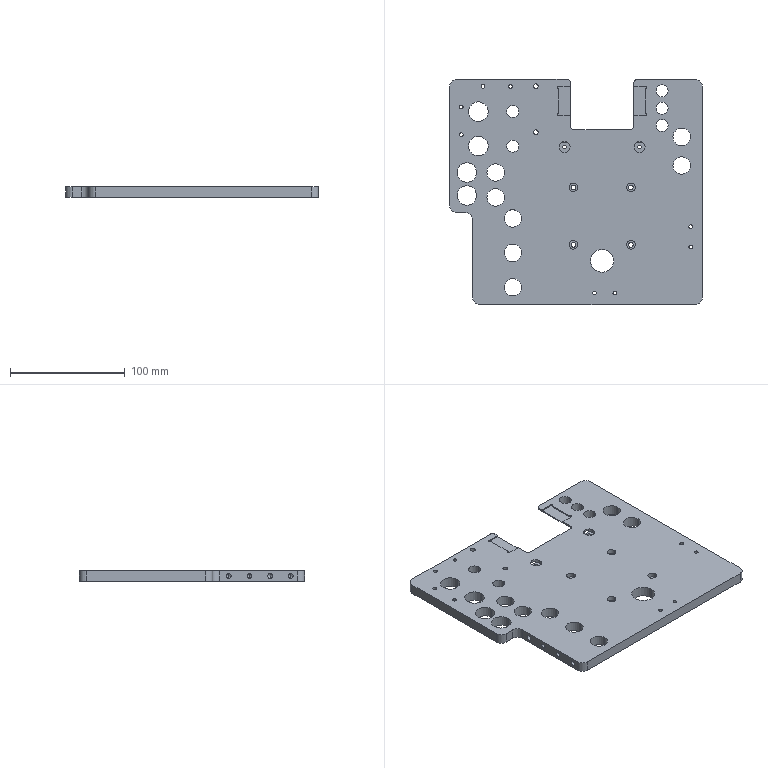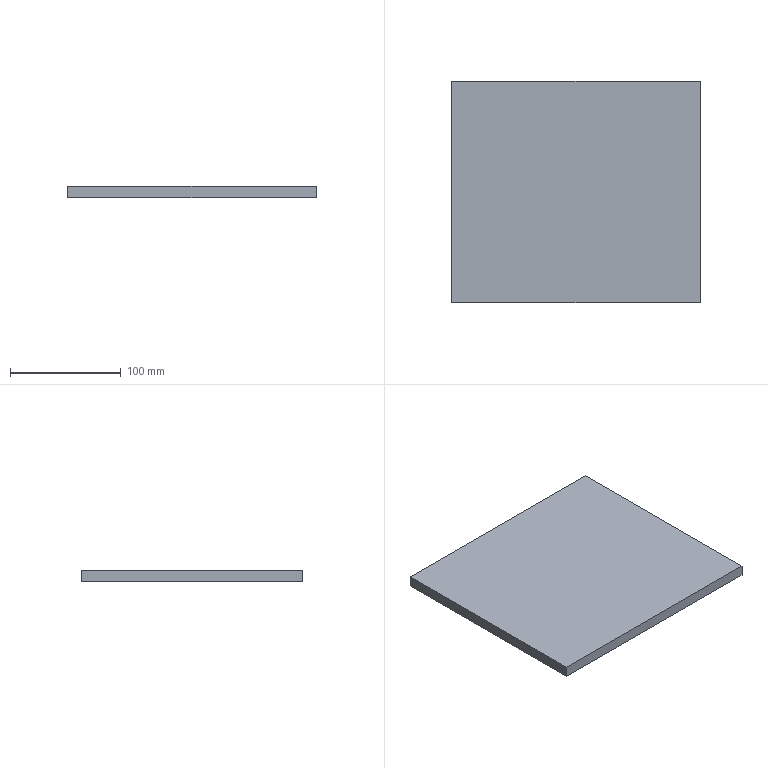CAM job | NX | 3-axis milling, drilling | part box 220 x 196 x 9 mm | stock box 224 x 200 x 10 mm
Tools:
number,name,description,diameter,corner_radius,flute_length,length,flutes
19,D80,Milling Tool-5 Parameters,80.0,0.0,50.0,75.0,2
1,D6A45,Milling Tool-5 Parameters,6.0,0.0,50.0,75.0,2
3,3.3ZT,Drilling Tool,3.3,0.0,35.0,50.0,2
4,4.2ZT,Drilling Tool,4.2,0.0,35.0,50.0,2
16,10.5ZT,Drilling Tool,10.5,0.0,35.0,50.0,2
15,D10,Milling Tool-5 Parameters,10.0,0.0,50.0,75.0,2
14,D10JING,Milling Tool-5 Parameters,10.0,0.0,50.0,75.0,2
12,D6,Milling Tool-5 Parameters,6.0,0.0,50.0,75.0,2
17,D2,Milling Tool-5 Parameters,2.0,0.0,50.0,75.0,2
18,D3,Milling Tool-5 Parameters,3.0,0.0,50.0,75.0,2
Operations:
program,operation,operation_type,tool,method,geometry_group,spindle_rpm,surface_speed,feed_per_tooth,feed_cut,feed_plunge,cut_length_mm,path_length_mm,cut_time_min,machine_time_min
1,FLOOR_WALL_COPY,VolumeBased25DMillingOperation,D80,METHOD,A,6500.0,1633.0,0.1154,1500.0,100.0,1399.997,1453.997,0.9333,0.9387
1,DRILLING_COPY_1,Operation,D6A45,METHOD,A,5000.0,94.0,0.035,350.0,0.0,132.0,1332.734,0.3771,0.4972
1,DRILLING_COPY_1_COPY_1_1_COPY_1,Operation,3.3ZT,METHOD,A,2000.0,34.0,0.05,200.0,0.0,144.914,783.73,0.7246,0.7885
1,DRILLING_COPY_1_COPY_1_1_COPY,Operation,4.2ZT,METHOD,A,2000.0,34.0,0.05,200.0,0.0,80.571,484.709,0.4029,0.4433
1,DRILLING_COPY_1_COPY_1_1_COPY_COPY,Operation,10.5ZT,METHOD,A,2000.0,34.0,0.05,200.0,0.0,283.127,1208.851,1.416,1.508
1,ZLEVEL_PROFILE,ZLevelMilling,D10,METHOD,A,9500.0,298.0,0.1684,3200.0,1000.0,8461.092,8526.492,2.676,2.683
1,ZLEVEL_PROFILE_COPY,ZLevelMilling,D10,METHOD,A,9500.0,298.0,0.1053,2000.0,1000.0,2799.662,4582.547,1.686,1.865
1,HOLE_MILLING,CylinderMilling,D6,METHOD,A,9500.0,179.0,0.0658,1250.0,100.0,385.956,987,0.3088,0.3689
1,FLOOR_WALL,VolumeBased25DMillingOperation,D6,METHOD,A,9500.0,179.0,0.0763,1450.0,100.0,368.116,682.737,0.2539,0.2853
1,ZLEVEL_PROFILE_2,ZLevelMilling,D6,METHOD,A,9500.0,179.0,0.0842,1600.0,100.0,58.786,241.589,0.0367,0.055
1,ZLEVEL_PROFILE_1,ZLevelMilling,D2,METHOD,A,9500.0,59.0,0.0579,1100.0,100.0,186.121,603.746,0.1692,0.211
1,ZLEVEL_PROFILE_COPY_1_COPY_COPY_1_COPY,ZLevelMilling,D10JING,METHOD,A,9500.0,298.0,0.0632,1200.0,1000.0,652.351,4005.362,0.559,0.8943
1,PLANAR_MILL_COPY_COPY_COPY_COPY_COPY_COPY_1_COPY_1,PlanarMilling,D6A45,METHOD,A,9500.0,179.0,0.0658,1250.0,100.0,2025.708,5066.1,1.621,1.925
1,ZLEVEL_PROFILE_COPY_1_COPY_COPY_1_COPY_COPY,ZLevelMilling,D10JING,METHOD,A,9500.0,298.0,0.0632,1200.0,1000.0,3723.615,3799.04,3.103,3.111
2,FLOOR_WALL_COPY_1,VolumeBased25DMillingOperation,D6,METHOD,B,9500.0,179.0,0.1158,2200.0,100.0,13194.974,14354.665,5.998,6.114
2,FLOOR_WALL_1,VolumeBased25DMillingOperation,D6,METHOD,B,9500.0,298.0,0.0658,1250.0,100.0,1177.533,1415.733,0.942,0.9658
2,HOLE_MILLING_COPY,CylinderMilling,D6,METHOD,B,9500.0,179.0,0.0658,1250.0,100.0,99.436,266.436,0.0795,0.0962
2,HOLE_MILLING_1,CylinderMilling,D3,METHOD,B,9500.0,89.0,0.0658,1250.0,100.0,826.724,1474.724,0.6614,0.7262
2,PLANAR_MILL_COPY_COPY_COPY_COPY_COPY_COPY_1_COPY_1_COPY,PlanarMilling,D6A45,METHOD,B,9500.0,179.0,0.0658,1250.0,100.0,2023.232,5520.6,1.619,1.968
2,ZLEVEL_PROFILE_COPY_1_COPY_COPY_1_COPY_COPY_1,ZLevelMilling,D6,METHOD,B,9500.0,298.0,0.0632,1200.0,1000.0,923.539,999.34,0.7701,0.7776